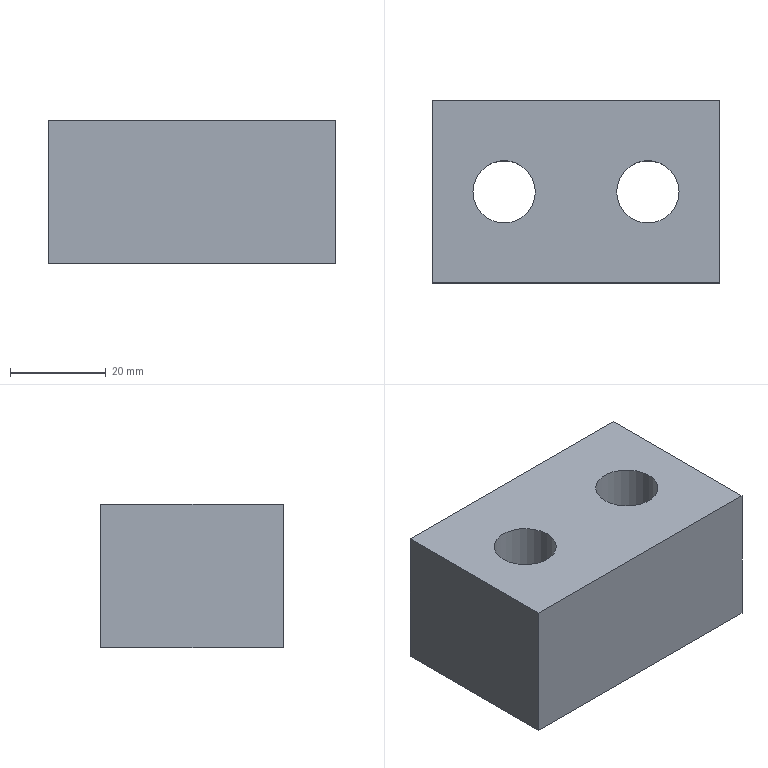Part | NX | features solid 2 | 1 solid | 12 faces | box 60 x 38 x 30 mm | volume 54993 mm3 | plane 8 | cylinder 4 | commonest cylinder face diameters 13 x2 20 x2
STEP:
#1=CARTESIAN_POINT('',(21.5,-50.,250.));
#2=VERTEX_POINT('',#1);
#3=CARTESIAN_POINT('',(15.,-50.,250.));
#4=DIRECTION('',(0.,0.,1.));
#5=DIRECTION('',(1.,0.,0.));
#6=AXIS2_PLACEMENT_3D('',#3,#4,#5);
#7=CIRCLE('',#6,6.5);
#8=EDGE_CURVE('',#2,#2,#7,.F.);
#9=ORIENTED_EDGE('',*,*,#8,.T.);
#10=EDGE_LOOP('',(#9));
#11=FACE_BOUND('',#10,.T.);
#12=CARTESIAN_POINT('',(-8.5,-50.,250.));
#13=VERTEX_POINT('',#12);
#14=CARTESIAN_POINT('',(-15.,-50.,250.));
#15=DIRECTION('',(0.,0.,1.));
#16=DIRECTION('',(1.,0.,0.));
#17=AXIS2_PLACEMENT_3D('',#14,#15,#16);
#18=CIRCLE('',#17,6.5);
#19=EDGE_CURVE('',#13,#13,#18,.F.);
#20=ORIENTED_EDGE('',*,*,#19,.T.);
#21=EDGE_LOOP('',(#20));
#22=FACE_BOUND('',#21,.T.);
#23=CARTESIAN_POINT('',(30.,-69.,250.));
#24=VERTEX_POINT('',#23);
#25=CARTESIAN_POINT('',(30.,-31.,250.));
#26=VERTEX_POINT('',#25);
#27=CARTESIAN_POINT('',(30.,-69.,250.));
#28=DIRECTION('',(0.,-1.,0.));
#29=VECTOR('',#28,1000.);
#30=LINE('',#27,#29);
#31=EDGE_CURVE('',#24,#26,#30,.F.);
#32=ORIENTED_EDGE('',*,*,#31,.T.);
#33=CARTESIAN_POINT('',(-30.,-31.,250.));
#34=VERTEX_POINT('',#33);
#35=CARTESIAN_POINT('',(30.,-31.,250.));
#36=DIRECTION('',(1.,0.,0.));
#37=VECTOR('',#36,1000.);
#38=LINE('',#35,#37);
#39=EDGE_CURVE('',#26,#34,#38,.F.);
#40=ORIENTED_EDGE('',*,*,#39,.T.);
#41=CARTESIAN_POINT('',(-30.,-69.,250.));
#42=VERTEX_POINT('',#41);
#43=CARTESIAN_POINT('',(-30.,-69.,250.));
#44=DIRECTION('',(0.,1.,0.));
#45=VECTOR('',#44,1000.);
#46=LINE('',#43,#45);
#47=EDGE_CURVE('',#42,#34,#46,.T.);
#48=ORIENTED_EDGE('',*,*,#47,.F.);
#49=CARTESIAN_POINT('',(30.,-69.,250.));
#50=DIRECTION('',(1.,0.,0.));
#51=VECTOR('',#50,1000.);
#52=LINE('',#49,#51);
#53=EDGE_CURVE('',#24,#42,#52,.F.);
#54=ORIENTED_EDGE('',*,*,#53,.F.);
#55=EDGE_LOOP('',(#32,#40,#48,#54));
#56=FACE_BOUND('',#55,.T.);
#57=CARTESIAN_POINT('',(30.,-69.,250.));
#58=DIRECTION('',(0.,0.,1.));
#59=DIRECTION('',(-1.,0.,0.));
#60=AXIS2_PLACEMENT_3D('',#57,#58,#59);
#61=PLANE('',#60);
#62=ADVANCED_FACE('',(#11,#22,#56),#61,.T.);
#63=ORIENTED_EDGE('',*,*,#47,.T.);
#64=CARTESIAN_POINT('',(-30.,-31.,220.));
#65=VERTEX_POINT('',#64);
#66=CARTESIAN_POINT('',(-30.,-31.,250.));
#67=DIRECTION('',(0.,0.,1.));
#68=VECTOR('',#67,1000.);
#69=LINE('',#66,#68);
#70=EDGE_CURVE('',#34,#65,#69,.F.);
#71=ORIENTED_EDGE('',*,*,#70,.T.);
#72=CARTESIAN_POINT('',(-30.,-69.,220.));
#73=VERTEX_POINT('',#72);
#74=CARTESIAN_POINT('',(-30.,-69.,220.));
#75=DIRECTION('',(0.,-1.,0.));
#76=VECTOR('',#75,1000.);
#77=LINE('',#74,#76);
#78=EDGE_CURVE('',#73,#65,#77,.F.);
#79=ORIENTED_EDGE('',*,*,#78,.F.);
#80=CARTESIAN_POINT('',(-30.,-69.,250.));
#81=DIRECTION('',(0.,0.,-1.));
#82=VECTOR('',#81,1000.);
#83=LINE('',#80,#82);
#84=EDGE_CURVE('',#42,#73,#83,.T.);
#85=ORIENTED_EDGE('',*,*,#84,.F.);
#86=EDGE_LOOP('',(#63,#71,#79,#85));
#87=FACE_BOUND('',#86,.T.);
#88=CARTESIAN_POINT('',(-30.,-69.,250.));
#89=DIRECTION('',(-1.,0.,0.));
#90=DIRECTION('',(0.,0.,-1.));
#91=AXIS2_PLACEMENT_3D('',#88,#89,#90);
#92=PLANE('',#91);
#93=ADVANCED_FACE('',(#87),#92,.T.);
#94=CARTESIAN_POINT('',(25.,-50.,220.));
#95=VERTEX_POINT('',#94);
#96=CARTESIAN_POINT('',(15.,-50.,220.));
#97=DIRECTION('',(0.,0.,1.));
#98=DIRECTION('',(1.,0.,0.));
#99=AXIS2_PLACEMENT_3D('',#96,#97,#98);
#100=CIRCLE('',#99,10.);
#101=EDGE_CURVE('',#95,#95,#100,.T.);
#102=ORIENTED_EDGE('',*,*,#101,.T.);
#103=EDGE_LOOP('',(#102));
#104=FACE_BOUND('',#103,.T.);
#105=CARTESIAN_POINT('',(-5.,-50.,220.));
#106=VERTEX_POINT('',#105);
#107=CARTESIAN_POINT('',(-15.,-50.,220.));
#108=DIRECTION('',(0.,0.,1.));
#109=DIRECTION('',(1.,0.,0.));
#110=AXIS2_PLACEMENT_3D('',#107,#108,#109);
#111=CIRCLE('',#110,10.);
#112=EDGE_CURVE('',#106,#106,#111,.T.);
#113=ORIENTED_EDGE('',*,*,#112,.T.);
#114=EDGE_LOOP('',(#113));
#115=FACE_BOUND('',#114,.T.);
#116=ORIENTED_EDGE('',*,*,#78,.T.);
#117=CARTESIAN_POINT('',(30.,-31.,220.));
#118=VERTEX_POINT('',#117);
#119=CARTESIAN_POINT('',(30.,-31.,220.));
#120=DIRECTION('',(-1.,0.,0.));
#121=VECTOR('',#120,1000.);
#122=LINE('',#119,#121);
#123=EDGE_CURVE('',#118,#65,#122,.T.);
#124=ORIENTED_EDGE('',*,*,#123,.F.);
#125=CARTESIAN_POINT('',(30.,-69.,220.));
#126=VERTEX_POINT('',#125);
#127=CARTESIAN_POINT('',(30.,-69.,220.));
#128=DIRECTION('',(0.,-1.,0.));
#129=VECTOR('',#128,1000.);
#130=LINE('',#127,#129);
#131=EDGE_CURVE('',#126,#118,#130,.F.);
#132=ORIENTED_EDGE('',*,*,#131,.F.);
#133=CARTESIAN_POINT('',(30.,-69.,220.));
#134=DIRECTION('',(-1.,0.,0.));
#135=VECTOR('',#134,1000.);
#136=LINE('',#133,#135);
#137=EDGE_CURVE('',#126,#73,#136,.T.);
#138=ORIENTED_EDGE('',*,*,#137,.T.);
#139=EDGE_LOOP('',(#116,#124,#132,#138));
#140=FACE_BOUND('',#139,.T.);
#141=CARTESIAN_POINT('',(30.,-69.,220.));
#142=DIRECTION('',(0.,0.,1.));
#143=DIRECTION('',(-1.,0.,0.));
#144=AXIS2_PLACEMENT_3D('',#141,#142,#143);
#145=PLANE('',#144);
#146=ADVANCED_FACE('',(#104,#115,#140),#145,.F.);
#147=CARTESIAN_POINT('',(30.,-69.,250.));
#148=DIRECTION('',(0.,0.,-1.));
#149=VECTOR('',#148,1000.);
#150=LINE('',#147,#149);
#151=EDGE_CURVE('',#24,#126,#150,.T.);
#152=ORIENTED_EDGE('',*,*,#151,.T.);
#153=ORIENTED_EDGE('',*,*,#131,.T.);
#154=CARTESIAN_POINT('',(30.,-31.,250.));
#155=DIRECTION('',(0.,0.,1.));
#156=VECTOR('',#155,1000.);
#157=LINE('',#154,#156);
#158=EDGE_CURVE('',#26,#118,#157,.F.);
#159=ORIENTED_EDGE('',*,*,#158,.F.);
#160=ORIENTED_EDGE('',*,*,#31,.F.);
#161=EDGE_LOOP('',(#152,#153,#159,#160));
#162=FACE_BOUND('',#161,.T.);
#163=CARTESIAN_POINT('',(30.,-69.,250.));
#164=DIRECTION('',(-1.,0.,0.));
#165=DIRECTION('',(0.,0.,-1.));
#166=AXIS2_PLACEMENT_3D('',#163,#164,#165);
#167=PLANE('',#166);
#168=ADVANCED_FACE('',(#162),#167,.F.);
#169=ORIENTED_EDGE('',*,*,#123,.T.);
#170=ORIENTED_EDGE('',*,*,#70,.F.);
#171=ORIENTED_EDGE('',*,*,#39,.F.);
#172=ORIENTED_EDGE('',*,*,#158,.T.);
#173=EDGE_LOOP('',(#169,#170,#171,#172));
#174=FACE_BOUND('',#173,.T.);
#175=CARTESIAN_POINT('',(30.,-31.,250.));
#176=DIRECTION('',(0.,-1.,0.));
#177=DIRECTION('',(0.,0.,1.));
#178=AXIS2_PLACEMENT_3D('',#175,#176,#177);
#179=PLANE('',#178);
#180=ADVANCED_FACE('',(#174),#179,.F.);
#181=ORIENTED_EDGE('',*,*,#137,.F.);
#182=ORIENTED_EDGE('',*,*,#151,.F.);
#183=ORIENTED_EDGE('',*,*,#53,.T.);
#184=ORIENTED_EDGE('',*,*,#84,.T.);
#185=EDGE_LOOP('',(#181,#182,#183,#184));
#186=FACE_BOUND('',#185,.T.);
#187=CARTESIAN_POINT('',(30.,-69.,250.));
#188=DIRECTION('',(0.,-1.,0.));
#189=DIRECTION('',(0.,0.,1.));
#190=AXIS2_PLACEMENT_3D('',#187,#188,#189);
#191=PLANE('',#190);
#192=ADVANCED_FACE('',(#186),#191,.T.);
#193=CARTESIAN_POINT('',(-8.5,-50.,235.));
#194=VERTEX_POINT('',#193);
#195=CARTESIAN_POINT('',(-15.,-50.,235.));
#196=DIRECTION('',(0.,0.,1.));
#197=DIRECTION('',(1.,0.,0.));
#198=AXIS2_PLACEMENT_3D('',#195,#196,#197);
#199=CIRCLE('',#198,6.5);
#200=EDGE_CURVE('',#194,#194,#199,.T.);
#201=ORIENTED_EDGE('',*,*,#200,.F.);
#202=EDGE_LOOP('',(#201));
#203=FACE_BOUND('',#202,.T.);
#204=ORIENTED_EDGE('',*,*,#19,.F.);
#205=EDGE_LOOP('',(#204));
#206=FACE_BOUND('',#205,.T.);
#207=CARTESIAN_POINT('',(-15.,-50.,270.));
#208=DIRECTION('',(0.,0.,1.));
#209=DIRECTION('',(1.,0.,0.));
#210=AXIS2_PLACEMENT_3D('',#207,#208,#209);
#211=CYLINDRICAL_SURFACE('',#210,6.5);
#212=ADVANCED_FACE('',(#203,#206),#211,.F.);
#213=ORIENTED_EDGE('',*,*,#200,.T.);
#214=EDGE_LOOP('',(#213));
#215=FACE_BOUND('',#214,.T.);
#216=CARTESIAN_POINT('',(-5.,-50.,235.));
#217=VERTEX_POINT('',#216);
#218=CARTESIAN_POINT('',(-15.,-50.,235.));
#219=DIRECTION('',(0.,0.,1.));
#220=DIRECTION('',(1.,0.,0.));
#221=AXIS2_PLACEMENT_3D('',#218,#219,#220);
#222=CIRCLE('',#221,10.);
#223=EDGE_CURVE('',#217,#217,#222,.T.);
#224=ORIENTED_EDGE('',*,*,#223,.F.);
#225=EDGE_LOOP('',(#224));
#226=FACE_BOUND('',#225,.T.);
#227=CARTESIAN_POINT('',(-15.,-50.,235.));
#228=DIRECTION('',(0.,0.,1.));
#229=DIRECTION('',(1.,0.,0.));
#230=AXIS2_PLACEMENT_3D('',#227,#228,#229);
#231=PLANE('',#230);
#232=ADVANCED_FACE('',(#215,#226),#231,.F.);
#233=ORIENTED_EDGE('',*,*,#223,.T.);
#234=EDGE_LOOP('',(#233));
#235=FACE_BOUND('',#234,.T.);
#236=ORIENTED_EDGE('',*,*,#112,.F.);
#237=EDGE_LOOP('',(#236));
#238=FACE_BOUND('',#237,.T.);
#239=CARTESIAN_POINT('',(-15.,-50.,220.));
#240=DIRECTION('',(0.,0.,1.));
#241=DIRECTION('',(1.,0.,0.));
#242=AXIS2_PLACEMENT_3D('',#239,#240,#241);
#243=CYLINDRICAL_SURFACE('',#242,10.);
#244=ADVANCED_FACE('',(#235,#238),#243,.F.);
#245=CARTESIAN_POINT('',(21.5,-50.,235.));
#246=VERTEX_POINT('',#245);
#247=CARTESIAN_POINT('',(15.,-50.,235.));
#248=DIRECTION('',(0.,0.,1.));
#249=DIRECTION('',(1.,0.,0.));
#250=AXIS2_PLACEMENT_3D('',#247,#248,#249);
#251=CIRCLE('',#250,6.5);
#252=EDGE_CURVE('',#246,#246,#251,.T.);
#253=ORIENTED_EDGE('',*,*,#252,.F.);
#254=EDGE_LOOP('',(#253));
#255=FACE_BOUND('',#254,.T.);
#256=ORIENTED_EDGE('',*,*,#8,.F.);
#257=EDGE_LOOP('',(#256));
#258=FACE_BOUND('',#257,.T.);
#259=CARTESIAN_POINT('',(15.,-50.,270.));
#260=DIRECTION('',(0.,0.,1.));
#261=DIRECTION('',(1.,0.,0.));
#262=AXIS2_PLACEMENT_3D('',#259,#260,#261);
#263=CYLINDRICAL_SURFACE('',#262,6.5);
#264=ADVANCED_FACE('',(#255,#258),#263,.F.);
#265=ORIENTED_EDGE('',*,*,#252,.T.);
#266=EDGE_LOOP('',(#265));
#267=FACE_BOUND('',#266,.T.);
#268=CARTESIAN_POINT('',(25.,-50.,235.));
#269=VERTEX_POINT('',#268);
#270=CARTESIAN_POINT('',(15.,-50.,235.));
#271=DIRECTION('',(0.,0.,1.));
#272=DIRECTION('',(1.,0.,0.));
#273=AXIS2_PLACEMENT_3D('',#270,#271,#272);
#274=CIRCLE('',#273,10.);
#275=EDGE_CURVE('',#269,#269,#274,.T.);
#276=ORIENTED_EDGE('',*,*,#275,.F.);
#277=EDGE_LOOP('',(#276));
#278=FACE_BOUND('',#277,.T.);
#279=CARTESIAN_POINT('',(15.,-50.,235.));
#280=DIRECTION('',(0.,0.,1.));
#281=DIRECTION('',(1.,0.,0.));
#282=AXIS2_PLACEMENT_3D('',#279,#280,#281);
#283=PLANE('',#282);
#284=ADVANCED_FACE('',(#267,#278),#283,.F.);
#285=ORIENTED_EDGE('',*,*,#275,.T.);
#286=EDGE_LOOP('',(#285));
#287=FACE_BOUND('',#286,.T.);
#288=ORIENTED_EDGE('',*,*,#101,.F.);
#289=EDGE_LOOP('',(#288));
#290=FACE_BOUND('',#289,.T.);
#291=CARTESIAN_POINT('',(15.,-50.,220.));
#292=DIRECTION('',(0.,0.,1.));
#293=DIRECTION('',(1.,0.,0.));
#294=AXIS2_PLACEMENT_3D('',#291,#292,#293);
#295=CYLINDRICAL_SURFACE('',#294,10.);
#296=ADVANCED_FACE('',(#287,#290),#295,.F.);
#297=CLOSED_SHELL('',(#62,#93,#146,#168,#180,#192,#212,#232,#244,#264,#284,#296));
#298=MANIFOLD_SOLID_BREP('',#297);
#299=(LENGTH_UNIT()NAMED_UNIT(*)SI_UNIT(.MILLI.,.METRE.));
#300=UNCERTAINTY_MEASURE_WITH_UNIT(LENGTH_MEASURE(0.00001),#299,'','');
#301=(NAMED_UNIT(*)PLANE_ANGLE_UNIT()SI_UNIT($,.RADIAN.));
#302=(NAMED_UNIT(*)SI_UNIT($,.STERADIAN.)SOLID_ANGLE_UNIT());
#303=(GEOMETRIC_REPRESENTATION_CONTEXT(3)GLOBAL_UNCERTAINTY_ASSIGNED_CONTEXT((#300))GLOBAL_UNIT_ASSIGNED_CONTEXT((#299,#301,#302))REPRESENTATION_CONTEXT('',''));
#304=ADVANCED_BREP_SHAPE_REPRESENTATION('',(#298),#303);